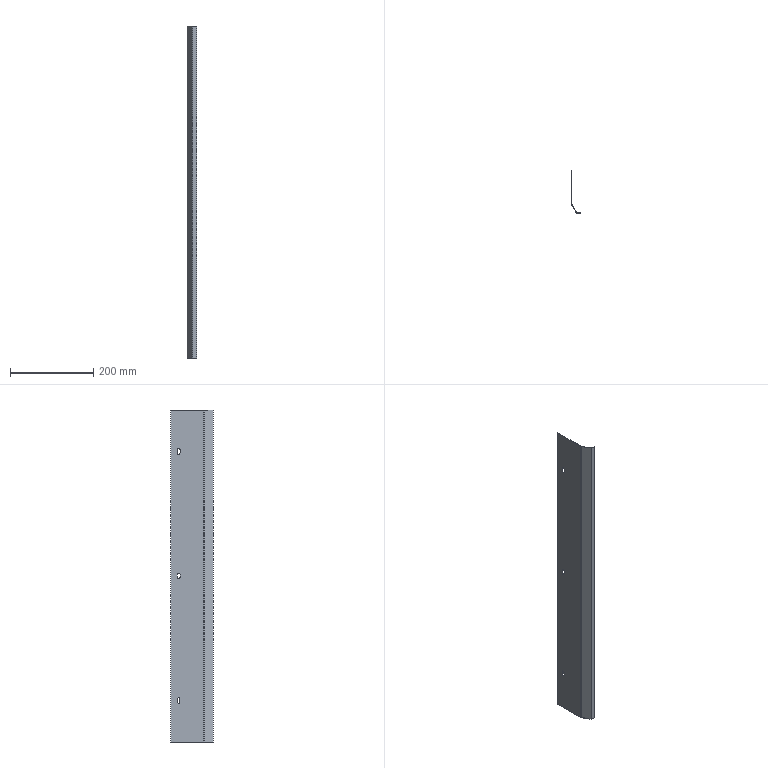Part | SolidWorks | features FlatPattern 1, ICE 1, SMBaseFlange 1, SheetMetal 1 | 1 solid | 37 faces | box 23.5 x 102.651 x 800 mm | volume 92335 mm3 | plane 24 | cylinder 13 | commonest cylinder face diameters 7 x6 6 x3 1 x2 3 x2
STEP:
#1=CARTESIAN_POINT('',(0.,-16.,-296.5));
#2=VERTEX_POINT('',#1);
#3=CARTESIAN_POINT('',(0.,-19.,-293.5));
#4=VERTEX_POINT('',#3);
#5=CARTESIAN_POINT('',(0.,-19.,-296.5));
#6=DIRECTION('',(1.,0.,0.));
#7=DIRECTION('',(0.,1.,0.));
#8=AXIS2_PLACEMENT_3D('',#5,#6,#7);
#9=CIRCLE('',#8,3.);
#10=EDGE_CURVE('',#2,#4,#9,.T.);
#11=ORIENTED_EDGE('',*,*,#10,.T.);
#12=CARTESIAN_POINT('',(-1.,-19.,-293.5));
#13=VERTEX_POINT('',#12);
#14=CARTESIAN_POINT('',(9.,-19.,-293.5));
#15=DIRECTION('',(-1.,0.,0.));
#16=VECTOR('',#15,1000.);
#17=LINE('',#14,#16);
#18=EDGE_CURVE('',#4,#13,#17,.T.);
#19=ORIENTED_EDGE('',*,*,#18,.T.);
#20=CARTESIAN_POINT('',(-1.,-16.,-296.5));
#21=VERTEX_POINT('',#20);
#22=CARTESIAN_POINT('',(-1.,-19.,-296.5));
#23=DIRECTION('',(-1.,0.,0.));
#24=DIRECTION('',(0.,0.,1.));
#25=AXIS2_PLACEMENT_3D('',#22,#23,#24);
#26=CIRCLE('',#25,3.);
#27=EDGE_CURVE('',#13,#21,#26,.T.);
#28=ORIENTED_EDGE('',*,*,#27,.T.);
#29=CARTESIAN_POINT('',(9.,-16.,-296.5));
#30=DIRECTION('',(-1.,0.,0.));
#31=VECTOR('',#30,1000.);
#32=LINE('',#29,#31);
#33=EDGE_CURVE('',#2,#21,#32,.T.);
#34=ORIENTED_EDGE('',*,*,#33,.F.);
#35=EDGE_LOOP('',(#11,#19,#28,#34));
#36=FACE_OUTER_BOUND('',#35,.T.);
#37=CARTESIAN_POINT('',(9.,-19.,-296.5));
#38=DIRECTION('',(-1.,0.,0.));
#39=DIRECTION('',(0.,0.,1.));
#40=AXIS2_PLACEMENT_3D('',#37,#38,#39);
#41=CYLINDRICAL_SURFACE('',#40,3.);
#42=ADVANCED_FACE('',(#36),#41,.F.);
#43=CARTESIAN_POINT('',(0.,-15.5,303.5));
#44=VERTEX_POINT('',#43);
#45=CARTESIAN_POINT('',(0.,-19.,307.));
#46=VERTEX_POINT('',#45);
#47=CARTESIAN_POINT('',(0.,-19.,303.5));
#48=DIRECTION('',(1.,0.,0.));
#49=DIRECTION('',(0.,1.,0.));
#50=AXIS2_PLACEMENT_3D('',#47,#48,#49);
#51=CIRCLE('',#50,3.5);
#52=EDGE_CURVE('',#44,#46,#51,.T.);
#53=ORIENTED_EDGE('',*,*,#52,.T.);
#54=CARTESIAN_POINT('',(-1.,-19.,307.));
#55=VERTEX_POINT('',#54);
#56=CARTESIAN_POINT('',(9.,-19.,307.));
#57=DIRECTION('',(-1.,0.,0.));
#58=VECTOR('',#57,1000.);
#59=LINE('',#56,#58);
#60=EDGE_CURVE('',#46,#55,#59,.T.);
#61=ORIENTED_EDGE('',*,*,#60,.T.);
#62=CARTESIAN_POINT('',(-1.,-15.5,303.5));
#63=VERTEX_POINT('',#62);
#64=CARTESIAN_POINT('',(-1.,-19.,303.5));
#65=DIRECTION('',(-1.,0.,0.));
#66=DIRECTION('',(0.,0.,1.));
#67=AXIS2_PLACEMENT_3D('',#64,#65,#66);
#68=CIRCLE('',#67,3.5);
#69=EDGE_CURVE('',#55,#63,#68,.T.);
#70=ORIENTED_EDGE('',*,*,#69,.T.);
#71=CARTESIAN_POINT('',(9.,-15.5,303.5));
#72=DIRECTION('',(-1.,0.,0.));
#73=VECTOR('',#72,1000.);
#74=LINE('',#71,#73);
#75=EDGE_CURVE('',#44,#63,#74,.T.);
#76=ORIENTED_EDGE('',*,*,#75,.F.);
#77=EDGE_LOOP('',(#53,#61,#70,#76));
#78=FACE_OUTER_BOUND('',#77,.T.);
#79=CARTESIAN_POINT('',(9.,-19.,303.5));
#80=DIRECTION('',(-1.,0.,0.));
#81=DIRECTION('',(0.,0.,1.));
#82=AXIS2_PLACEMENT_3D('',#79,#80,#81);
#83=CYLINDRICAL_SURFACE('',#82,3.5);
#84=ADVANCED_FACE('',(#78),#83,.F.);
#85=CARTESIAN_POINT('',(0.,-15.5,3.5));
#86=VERTEX_POINT('',#85);
#87=CARTESIAN_POINT('',(0.,-19.,7.));
#88=VERTEX_POINT('',#87);
#89=CARTESIAN_POINT('',(0.,-19.,3.5));
#90=DIRECTION('',(1.,0.,0.));
#91=DIRECTION('',(0.,1.,0.));
#92=AXIS2_PLACEMENT_3D('',#89,#90,#91);
#93=CIRCLE('',#92,3.5);
#94=EDGE_CURVE('',#86,#88,#93,.T.);
#95=ORIENTED_EDGE('',*,*,#94,.T.);
#96=CARTESIAN_POINT('',(-1.,-19.,7.));
#97=VERTEX_POINT('',#96);
#98=CARTESIAN_POINT('',(9.,-19.,7.));
#99=DIRECTION('',(-1.,0.,0.));
#100=VECTOR('',#99,1000.);
#101=LINE('',#98,#100);
#102=EDGE_CURVE('',#88,#97,#101,.T.);
#103=ORIENTED_EDGE('',*,*,#102,.T.);
#104=CARTESIAN_POINT('',(-1.,-15.5,3.5));
#105=VERTEX_POINT('',#104);
#106=CARTESIAN_POINT('',(-1.,-19.,3.5));
#107=DIRECTION('',(-1.,0.,0.));
#108=DIRECTION('',(0.,0.,1.));
#109=AXIS2_PLACEMENT_3D('',#106,#107,#108);
#110=CIRCLE('',#109,3.5);
#111=EDGE_CURVE('',#97,#105,#110,.T.);
#112=ORIENTED_EDGE('',*,*,#111,.T.);
#113=CARTESIAN_POINT('',(9.,-15.5,3.5));
#114=DIRECTION('',(-1.,0.,0.));
#115=VECTOR('',#114,1000.);
#116=LINE('',#113,#115);
#117=EDGE_CURVE('',#86,#105,#116,.T.);
#118=ORIENTED_EDGE('',*,*,#117,.F.);
#119=EDGE_LOOP('',(#95,#103,#112,#118));
#120=FACE_OUTER_BOUND('',#119,.T.);
#121=CARTESIAN_POINT('',(9.,-19.,3.5));
#122=DIRECTION('',(-1.,0.,0.));
#123=DIRECTION('',(0.,0.,1.));
#124=AXIS2_PLACEMENT_3D('',#121,#122,#123);
#125=CYLINDRICAL_SURFACE('',#124,3.5);
#126=ADVANCED_FACE('',(#120),#125,.F.);
#127=CARTESIAN_POINT('',(0.06699,-80.116,400.));
#128=VERTEX_POINT('',#127);
#129=CARTESIAN_POINT('',(-0.799,-80.616,400.));
#130=VERTEX_POINT('',#129);
#131=CARTESIAN_POINT('',(0.06699,-80.116,400.));
#132=DIRECTION('',(-0.866,-0.5,0.));
#133=VECTOR('',#132,1000.);
#134=LINE('',#131,#133);
#135=EDGE_CURVE('',#128,#130,#134,.T.);
#136=ORIENTED_EDGE('',*,*,#135,.F.);
#137=CARTESIAN_POINT('',(0.,-79.866,400.));
#138=VERTEX_POINT('',#137);
#139=CARTESIAN_POINT('',(0.5,-79.866,400.));
#140=DIRECTION('',(0.,0.,1.));
#141=DIRECTION('',(-1.,0.,0.));
#142=AXIS2_PLACEMENT_3D('',#139,#140,#141);
#143=CIRCLE('',#142,0.5);
#144=EDGE_CURVE('',#138,#128,#143,.T.);
#145=ORIENTED_EDGE('',*,*,#144,.F.);
#146=CARTESIAN_POINT('',(-1.,-79.866,400.));
#147=VERTEX_POINT('',#146);
#148=CARTESIAN_POINT('',(-1.,-79.866,400.));
#149=DIRECTION('',(1.,0.,0.));
#150=VECTOR('',#149,1000.);
#151=LINE('',#148,#150);
#152=EDGE_CURVE('',#147,#138,#151,.T.);
#153=ORIENTED_EDGE('',*,*,#152,.F.);
#154=CARTESIAN_POINT('',(0.5,-79.866,400.));
#155=DIRECTION('',(0.,0.,1.));
#156=DIRECTION('',(1.,0.,0.));
#157=AXIS2_PLACEMENT_3D('',#154,#155,#156);
#158=CIRCLE('',#157,1.5);
#159=EDGE_CURVE('',#147,#130,#158,.T.);
#160=ORIENTED_EDGE('',*,*,#159,.T.);
#161=EDGE_LOOP('',(#136,#145,#153,#160));
#162=FACE_OUTER_BOUND('',#161,.T.);
#163=CARTESIAN_POINT('',(0.06699,-80.116,400.));
#164=DIRECTION('',(0.,0.,1.));
#165=DIRECTION('',(1.,0.,0.));
#166=AXIS2_PLACEMENT_3D('',#163,#164,#165);
#167=PLANE('',#166);
#168=ADVANCED_FACE('',(#162),#167,.T.);
#169=CARTESIAN_POINT('',(12.356,-101.401,400.));
#170=VERTEX_POINT('',#169);
#171=CARTESIAN_POINT('',(0.,-80.,400.));
#172=DIRECTION('',(0.5,-0.866,0.));
#173=VECTOR('',#172,1000.);
#174=LINE('',#171,#173);
#175=EDGE_CURVE('',#128,#170,#174,.T.);
#176=ORIENTED_EDGE('',*,*,#175,.F.);
#177=ORIENTED_EDGE('',*,*,#135,.T.);
#178=CARTESIAN_POINT('',(11.49,-101.901,400.));
#179=VERTEX_POINT('',#178);
#180=CARTESIAN_POINT('',(-0.866,-80.5,400.));
#181=DIRECTION('',(0.5,-0.866,0.));
#182=VECTOR('',#181,1000.);
#183=LINE('',#180,#182);
#184=EDGE_CURVE('',#130,#179,#183,.T.);
#185=ORIENTED_EDGE('',*,*,#184,.T.);
#186=CARTESIAN_POINT('',(11.49,-101.901,400.));
#187=DIRECTION('',(0.866,0.5,0.));
#188=VECTOR('',#187,1000.);
#189=LINE('',#186,#188);
#190=EDGE_CURVE('',#179,#170,#189,.T.);
#191=ORIENTED_EDGE('',*,*,#190,.T.);
#192=EDGE_LOOP('',(#176,#177,#185,#191));
#193=FACE_OUTER_BOUND('',#192,.T.);
#194=CARTESIAN_POINT('',(-1.,-79.866,400.));
#195=DIRECTION('',(0.,0.,1.));
#196=DIRECTION('',(1.,0.,0.));
#197=AXIS2_PLACEMENT_3D('',#194,#195,#196);
#198=PLANE('',#197);
#199=ADVANCED_FACE('',(#193),#198,.T.);
#200=CARTESIAN_POINT('',(0.,-79.866,-400.));
#201=VERTEX_POINT('',#200);
#202=CARTESIAN_POINT('',(-1.,-79.866,-400.));
#203=VERTEX_POINT('',#202);
#204=CARTESIAN_POINT('',(0.,-79.866,-400.));
#205=DIRECTION('',(-1.,0.,0.));
#206=VECTOR('',#205,1000.);
#207=LINE('',#204,#206);
#208=EDGE_CURVE('',#201,#203,#207,.T.);
#209=ORIENTED_EDGE('',*,*,#208,.F.);
#210=CARTESIAN_POINT('',(0.06699,-80.116,-400.));
#211=VERTEX_POINT('',#210);
#212=CARTESIAN_POINT('',(0.5,-79.866,-400.));
#213=DIRECTION('',(0.,0.,1.));
#214=DIRECTION('',(-1.,0.,0.));
#215=AXIS2_PLACEMENT_3D('',#212,#213,#214);
#216=CIRCLE('',#215,0.5);
#217=EDGE_CURVE('',#201,#211,#216,.T.);
#218=ORIENTED_EDGE('',*,*,#217,.T.);
#219=CARTESIAN_POINT('',(-0.799,-80.616,-400.));
#220=VERTEX_POINT('',#219);
#221=CARTESIAN_POINT('',(-0.799,-80.616,-400.));
#222=DIRECTION('',(0.866,0.5,0.));
#223=VECTOR('',#222,1000.);
#224=LINE('',#221,#223);
#225=EDGE_CURVE('',#220,#211,#224,.T.);
#226=ORIENTED_EDGE('',*,*,#225,.F.);
#227=CARTESIAN_POINT('',(0.5,-79.866,-400.));
#228=DIRECTION('',(0.,0.,1.));
#229=DIRECTION('',(1.,0.,0.));
#230=AXIS2_PLACEMENT_3D('',#227,#228,#229);
#231=CIRCLE('',#230,1.5);
#232=EDGE_CURVE('',#203,#220,#231,.T.);
#233=ORIENTED_EDGE('',*,*,#232,.F.);
#234=EDGE_LOOP('',(#209,#218,#226,#233));
#235=FACE_OUTER_BOUND('',#234,.T.);
#236=CARTESIAN_POINT('',(0.,-79.866,-400.));
#237=DIRECTION('',(0.,0.,-1.));
#238=DIRECTION('',(-1.,0.,0.));
#239=AXIS2_PLACEMENT_3D('',#236,#237,#238);
#240=PLANE('',#239);
#241=ADVANCED_FACE('',(#235),#240,.T.);
#242=CARTESIAN_POINT('',(0.,0.,-400.));
#243=VERTEX_POINT('',#242);
#244=CARTESIAN_POINT('',(0.,0.,-400.));
#245=DIRECTION('',(0.,-1.,0.));
#246=VECTOR('',#245,1000.);
#247=LINE('',#244,#246);
#248=EDGE_CURVE('',#243,#201,#247,.T.);
#249=ORIENTED_EDGE('',*,*,#248,.T.);
#250=ORIENTED_EDGE('',*,*,#208,.T.);
#251=CARTESIAN_POINT('',(-1.,0.,-400.));
#252=VERTEX_POINT('',#251);
#253=CARTESIAN_POINT('',(-1.,0.,-400.));
#254=DIRECTION('',(0.,-1.,0.));
#255=VECTOR('',#254,1000.);
#256=LINE('',#253,#255);
#257=EDGE_CURVE('',#252,#203,#256,.T.);
#258=ORIENTED_EDGE('',*,*,#257,.F.);
#259=CARTESIAN_POINT('',(-1.,0.,-400.));
#260=DIRECTION('',(1.,0.,0.));
#261=VECTOR('',#260,1000.);
#262=LINE('',#259,#261);
#263=EDGE_CURVE('',#252,#243,#262,.T.);
#264=ORIENTED_EDGE('',*,*,#263,.T.);
#265=EDGE_LOOP('',(#249,#250,#258,#264));
#266=FACE_OUTER_BOUND('',#265,.T.);
#267=CARTESIAN_POINT('',(-0.799,-80.616,-400.));
#268=DIRECTION('',(0.,0.,-1.));
#269=DIRECTION('',(-1.,0.,0.));
#270=AXIS2_PLACEMENT_3D('',#267,#268,#269);
#271=PLANE('',#270);
#272=ADVANCED_FACE('',(#266),#271,.T.);
#273=CARTESIAN_POINT('',(12.789,-101.651,400.));
#274=VERTEX_POINT('',#273);
#275=CARTESIAN_POINT('',(12.789,-102.651,400.));
#276=VERTEX_POINT('',#275);
#277=CARTESIAN_POINT('',(12.789,-101.651,400.));
#278=DIRECTION('',(0.,-1.,0.));
#279=VECTOR('',#278,1000.);
#280=LINE('',#277,#279);
#281=EDGE_CURVE('',#274,#276,#280,.T.);
#282=ORIENTED_EDGE('',*,*,#281,.F.);
#283=CARTESIAN_POINT('',(12.789,-101.151,400.));
#284=DIRECTION('',(0.,0.,1.));
#285=DIRECTION('',(-1.,0.,0.));
#286=AXIS2_PLACEMENT_3D('',#283,#284,#285);
#287=CIRCLE('',#286,0.5);
#288=EDGE_CURVE('',#170,#274,#287,.T.);
#289=ORIENTED_EDGE('',*,*,#288,.F.);
#290=ORIENTED_EDGE('',*,*,#190,.F.);
#291=CARTESIAN_POINT('',(12.789,-101.151,400.));
#292=DIRECTION('',(0.,0.,1.));
#293=DIRECTION('',(1.,0.,0.));
#294=AXIS2_PLACEMENT_3D('',#291,#292,#293);
#295=CIRCLE('',#294,1.5);
#296=EDGE_CURVE('',#179,#276,#295,.T.);
#297=ORIENTED_EDGE('',*,*,#296,.T.);
#298=EDGE_LOOP('',(#282,#289,#290,#297));
#299=FACE_OUTER_BOUND('',#298,.T.);
#300=CARTESIAN_POINT('',(12.789,-101.651,400.));
#301=DIRECTION('',(0.,0.,1.));
#302=DIRECTION('',(1.,0.,0.));
#303=AXIS2_PLACEMENT_3D('',#300,#301,#302);
#304=PLANE('',#303);
#305=ADVANCED_FACE('',(#299),#304,.T.);
#306=CARTESIAN_POINT('',(22.5,-101.651,400.));
#307=VERTEX_POINT('',#306);
#308=CARTESIAN_POINT('',(12.5,-101.651,400.));
#309=DIRECTION('',(1.,0.,0.));
#310=VECTOR('',#309,1000.);
#311=LINE('',#308,#310);
#312=EDGE_CURVE('',#274,#307,#311,.T.);
#313=ORIENTED_EDGE('',*,*,#312,.F.);
#314=ORIENTED_EDGE('',*,*,#281,.T.);
#315=CARTESIAN_POINT('',(22.5,-102.651,400.));
#316=VERTEX_POINT('',#315);
#317=CARTESIAN_POINT('',(12.5,-102.651,400.));
#318=DIRECTION('',(1.,0.,0.));
#319=VECTOR('',#318,1000.);
#320=LINE('',#317,#319);
#321=EDGE_CURVE('',#276,#316,#320,.T.);
#322=ORIENTED_EDGE('',*,*,#321,.T.);
#323=CARTESIAN_POINT('',(22.5,-101.651,400.));
#324=DIRECTION('',(0.,-1.,0.));
#325=VECTOR('',#324,1000.);
#326=LINE('',#323,#325);
#327=EDGE_CURVE('',#307,#316,#326,.T.);
#328=ORIENTED_EDGE('',*,*,#327,.F.);
#329=EDGE_LOOP('',(#313,#314,#322,#328));
#330=FACE_OUTER_BOUND('',#329,.T.);
#331=CARTESIAN_POINT('',(11.49,-101.901,400.));
#332=DIRECTION('',(0.,0.,1.));
#333=DIRECTION('',(1.,0.,0.));
#334=AXIS2_PLACEMENT_3D('',#331,#332,#333);
#335=PLANE('',#334);
#336=ADVANCED_FACE('',(#330),#335,.T.);
#337=CARTESIAN_POINT('',(12.356,-101.401,-400.));
#338=VERTEX_POINT('',#337);
#339=CARTESIAN_POINT('',(11.49,-101.901,-400.));
#340=VERTEX_POINT('',#339);
#341=CARTESIAN_POINT('',(12.356,-101.401,-400.));
#342=DIRECTION('',(-0.866,-0.5,0.));
#343=VECTOR('',#342,1000.);
#344=LINE('',#341,#343);
#345=EDGE_CURVE('',#338,#340,#344,.T.);
#346=ORIENTED_EDGE('',*,*,#345,.F.);
#347=CARTESIAN_POINT('',(12.789,-101.651,-400.));
#348=VERTEX_POINT('',#347);
#349=CARTESIAN_POINT('',(12.789,-101.151,-400.));
#350=DIRECTION('',(0.,0.,1.));
#351=DIRECTION('',(-1.,0.,0.));
#352=AXIS2_PLACEMENT_3D('',#349,#350,#351);
#353=CIRCLE('',#352,0.5);
#354=EDGE_CURVE('',#338,#348,#353,.T.);
#355=ORIENTED_EDGE('',*,*,#354,.T.);
#356=CARTESIAN_POINT('',(12.789,-102.651,-400.));
#357=VERTEX_POINT('',#356);
#358=CARTESIAN_POINT('',(12.789,-102.651,-400.));
#359=DIRECTION('',(0.,1.,0.));
#360=VECTOR('',#359,1000.);
#361=LINE('',#358,#360);
#362=EDGE_CURVE('',#357,#348,#361,.T.);
#363=ORIENTED_EDGE('',*,*,#362,.F.);
#364=CARTESIAN_POINT('',(12.789,-101.151,-400.));
#365=DIRECTION('',(0.,0.,1.));
#366=DIRECTION('',(1.,0.,0.));
#367=AXIS2_PLACEMENT_3D('',#364,#365,#366);
#368=CIRCLE('',#367,1.5);
#369=EDGE_CURVE('',#340,#357,#368,.T.);
#370=ORIENTED_EDGE('',*,*,#369,.F.);
#371=EDGE_LOOP('',(#346,#355,#363,#370));
#372=FACE_OUTER_BOUND('',#371,.T.);
#373=CARTESIAN_POINT('',(12.356,-101.401,-400.));
#374=DIRECTION('',(0.,0.,-1.));
#375=DIRECTION('',(-1.,0.,0.));
#376=AXIS2_PLACEMENT_3D('',#373,#374,#375);
#377=PLANE('',#376);
#378=ADVANCED_FACE('',(#372),#377,.T.);
#379=CARTESIAN_POINT('',(0.,-80.,-400.));
#380=DIRECTION('',(0.5,-0.866,0.));
#381=VECTOR('',#380,1000.);
#382=LINE('',#379,#381);
#383=EDGE_CURVE('',#211,#338,#382,.T.);
#384=ORIENTED_EDGE('',*,*,#383,.T.);
#385=ORIENTED_EDGE('',*,*,#345,.T.);
#386=CARTESIAN_POINT('',(-0.866,-80.5,-400.));
#387=DIRECTION('',(0.5,-0.866,0.));
#388=VECTOR('',#387,1000.);
#389=LINE('',#386,#388);
#390=EDGE_CURVE('',#220,#340,#389,.T.);
#391=ORIENTED_EDGE('',*,*,#390,.F.);
#392=ORIENTED_EDGE('',*,*,#225,.T.);
#393=EDGE_LOOP('',(#384,#385,#391,#392));
#394=FACE_OUTER_BOUND('',#393,.T.);
#395=CARTESIAN_POINT('',(12.789,-102.651,-400.));
#396=DIRECTION('',(0.,0.,-1.));
#397=DIRECTION('',(-1.,0.,0.));
#398=AXIS2_PLACEMENT_3D('',#395,#396,#397);
#399=PLANE('',#398);
#400=ADVANCED_FACE('',(#394),#399,.T.);
#401=CARTESIAN_POINT('',(22.5,-102.651,-400.));
#402=VERTEX_POINT('',#401);
#403=CARTESIAN_POINT('',(12.5,-102.651,-400.));
#404=DIRECTION('',(1.,0.,0.));
#405=VECTOR('',#404,1000.);
#406=LINE('',#403,#405);
#407=EDGE_CURVE('',#357,#402,#406,.T.);
#408=ORIENTED_EDGE('',*,*,#407,.T.);
#409=CARTESIAN_POINT('',(22.5,-102.651,400.));
#410=DIRECTION('',(0.,0.,-1.));
#411=VECTOR('',#410,1000.);
#412=LINE('',#409,#411);
#413=EDGE_CURVE('',#316,#402,#412,.T.);
#414=ORIENTED_EDGE('',*,*,#413,.F.);
#415=ORIENTED_EDGE('',*,*,#321,.F.);
#416=CARTESIAN_POINT('',(12.789,-102.651,400.));
#417=DIRECTION('',(0.,0.,-1.));
#418=VECTOR('',#417,1000.);
#419=LINE('',#416,#418);
#420=EDGE_CURVE('',#276,#357,#419,.T.);
#421=ORIENTED_EDGE('',*,*,#420,.T.);
#422=EDGE_LOOP('',(#408,#414,#415,#421));
#423=FACE_OUTER_BOUND('',#422,.T.);
#424=CARTESIAN_POINT('',(12.5,-102.651,400.));
#425=DIRECTION('',(0.,1.,0.));
#426=DIRECTION('',(0.,0.,1.));
#427=AXIS2_PLACEMENT_3D('',#424,#425,#426);
#428=PLANE('',#427);
#429=ADVANCED_FACE('',(#423),#428,.F.);
#430=CARTESIAN_POINT('',(22.5,-101.651,-400.));
#431=VERTEX_POINT('',#430);
#432=CARTESIAN_POINT('',(22.5,-101.651,-400.));
#433=DIRECTION('',(0.,-1.,0.));
#434=VECTOR('',#433,1000.);
#435=LINE('',#432,#434);
#436=EDGE_CURVE('',#431,#402,#435,.T.);
#437=ORIENTED_EDGE('',*,*,#436,.F.);
#438=CARTESIAN_POINT('',(22.5,-101.651,400.));
#439=DIRECTION('',(0.,0.,-1.));
#440=VECTOR('',#439,1000.);
#441=LINE('',#438,#440);
#442=EDGE_CURVE('',#307,#431,#441,.T.);
#443=ORIENTED_EDGE('',*,*,#442,.F.);
#444=ORIENTED_EDGE('',*,*,#327,.T.);
#445=ORIENTED_EDGE('',*,*,#413,.T.);
#446=EDGE_LOOP('',(#437,#443,#444,#445));
#447=FACE_OUTER_BOUND('',#446,.T.);
#448=CARTESIAN_POINT('',(22.5,-101.651,400.));
#449=DIRECTION('',(1.,0.,0.));
#450=DIRECTION('',(0.,0.,-1.));
#451=AXIS2_PLACEMENT_3D('',#448,#449,#450);
#452=PLANE('',#451);
#453=ADVANCED_FACE('',(#447),#452,.T.);
#454=CARTESIAN_POINT('',(12.5,-101.651,-400.));
#455=DIRECTION('',(1.,0.,0.));
#456=VECTOR('',#455,1000.);
#457=LINE('',#454,#456);
#458=EDGE_CURVE('',#348,#431,#457,.T.);
#459=ORIENTED_EDGE('',*,*,#458,.F.);
#460=CARTESIAN_POINT('',(12.789,-101.651,400.));
#461=DIRECTION('',(0.,0.,-1.));
#462=VECTOR('',#461,1000.);
#463=LINE('',#460,#462);
#464=EDGE_CURVE('',#274,#348,#463,.T.);
#465=ORIENTED_EDGE('',*,*,#464,.F.);
#466=ORIENTED_EDGE('',*,*,#312,.T.);
#467=ORIENTED_EDGE('',*,*,#442,.T.);
#468=EDGE_LOOP('',(#459,#465,#466,#467));
#469=FACE_OUTER_BOUND('',#468,.T.);
#470=CARTESIAN_POINT('',(12.5,-101.651,400.));
#471=DIRECTION('',(0.,1.,0.));
#472=DIRECTION('',(0.,0.,1.));
#473=AXIS2_PLACEMENT_3D('',#470,#471,#472);
#474=PLANE('',#473);
#475=ADVANCED_FACE('',(#469),#474,.T.);
#476=ORIENTED_EDGE('',*,*,#354,.F.);
#477=CARTESIAN_POINT('',(12.356,-101.401,400.));
#478=DIRECTION('',(0.,0.,-1.));
#479=VECTOR('',#478,1000.);
#480=LINE('',#477,#479);
#481=EDGE_CURVE('',#170,#338,#480,.T.);
#482=ORIENTED_EDGE('',*,*,#481,.F.);
#483=ORIENTED_EDGE('',*,*,#288,.T.);
#484=ORIENTED_EDGE('',*,*,#464,.T.);
#485=EDGE_LOOP('',(#476,#482,#483,#484));
#486=FACE_OUTER_BOUND('',#485,.T.);
#487=CARTESIAN_POINT('',(12.789,-101.151,400.));
#488=DIRECTION('',(0.,0.,-1.));
#489=DIRECTION('',(-1.,0.,0.));
#490=AXIS2_PLACEMENT_3D('',#487,#488,#489);
#491=CYLINDRICAL_SURFACE('',#490,0.5);
#492=ADVANCED_FACE('',(#486),#491,.F.);
#493=ORIENTED_EDGE('',*,*,#383,.F.);
#494=CARTESIAN_POINT('',(0.06699,-80.116,400.));
#495=DIRECTION('',(0.,0.,-1.));
#496=VECTOR('',#495,1000.);
#497=LINE('',#494,#496);
#498=EDGE_CURVE('',#128,#211,#497,.T.);
#499=ORIENTED_EDGE('',*,*,#498,.F.);
#500=ORIENTED_EDGE('',*,*,#175,.T.);
#501=ORIENTED_EDGE('',*,*,#481,.T.);
#502=EDGE_LOOP('',(#493,#499,#500,#501));
#503=FACE_OUTER_BOUND('',#502,.T.);
#504=CARTESIAN_POINT('',(0.,-80.,400.));
#505=DIRECTION('',(0.866,0.5,0.));
#506=DIRECTION('',(-0.5,0.866,0.));
#507=AXIS2_PLACEMENT_3D('',#504,#505,#506);
#508=PLANE('',#507);
#509=ADVANCED_FACE('',(#503),#508,.T.);
#510=ORIENTED_EDGE('',*,*,#217,.F.);
#511=CARTESIAN_POINT('',(0.,-79.866,400.));
#512=DIRECTION('',(0.,0.,-1.));
#513=VECTOR('',#512,1000.);
#514=LINE('',#511,#513);
#515=EDGE_CURVE('',#138,#201,#514,.T.);
#516=ORIENTED_EDGE('',*,*,#515,.F.);
#517=ORIENTED_EDGE('',*,*,#144,.T.);
#518=ORIENTED_EDGE('',*,*,#498,.T.);
#519=EDGE_LOOP('',(#510,#516,#517,#518));
#520=FACE_OUTER_BOUND('',#519,.T.);
#521=CARTESIAN_POINT('',(0.5,-79.866,400.));
#522=DIRECTION('',(0.,0.,-1.));
#523=DIRECTION('',(-1.,0.,0.));
#524=AXIS2_PLACEMENT_3D('',#521,#522,#523);
#525=CYLINDRICAL_SURFACE('',#524,0.5);
#526=ADVANCED_FACE('',(#520),#525,.F.);
#527=CARTESIAN_POINT('',(0.,-22.,-303.5));
#528=VERTEX_POINT('',#527);
#529=CARTESIAN_POINT('',(0.,-16.,-303.5));
#530=VERTEX_POINT('',#529);
#531=CARTESIAN_POINT('',(0.,-19.,-303.5));
#532=DIRECTION('',(1.,0.,0.));
#533=DIRECTION('',(0.,1.,0.));
#534=AXIS2_PLACEMENT_3D('',#531,#532,#533);
#535=CIRCLE('',#534,3.);
#536=EDGE_CURVE('',#528,#530,#535,.T.);
#537=ORIENTED_EDGE('',*,*,#536,.F.);
#538=CARTESIAN_POINT('',(0.,-22.,-296.5));
#539=VERTEX_POINT('',#538);
#540=CARTESIAN_POINT('',(0.,-22.,400.));
#541=DIRECTION('',(0.,0.,-1.));
#542=VECTOR('',#541,1000.);
#543=LINE('',#540,#542);
#544=EDGE_CURVE('',#539,#528,#543,.T.);
#545=ORIENTED_EDGE('',*,*,#544,.F.);
#546=CARTESIAN_POINT('',(0.,-19.,-296.5));
#547=DIRECTION('',(1.,0.,0.));
#548=DIRECTION('',(0.,1.,0.));
#549=AXIS2_PLACEMENT_3D('',#546,#547,#548);
#550=CIRCLE('',#549,3.);
#551=EDGE_CURVE('',#4,#539,#550,.T.);
#552=ORIENTED_EDGE('',*,*,#551,.F.);
#553=ORIENTED_EDGE('',*,*,#10,.F.);
#554=CARTESIAN_POINT('',(0.,-16.,400.));
#555=DIRECTION('',(0.,0.,1.));
#556=VECTOR('',#555,1000.);
#557=LINE('',#554,#556);
#558=EDGE_CURVE('',#530,#2,#557,.T.);
#559=ORIENTED_EDGE('',*,*,#558,.F.);
#560=EDGE_LOOP('',(#537,#545,#552,#553,#559));
#561=FACE_BOUND('',#560,.T.);
#562=CARTESIAN_POINT('',(0.,-22.5,296.5));
#563=VERTEX_POINT('',#562);
#564=CARTESIAN_POINT('',(0.,-15.5,296.5));
#565=VERTEX_POINT('',#564);
#566=CARTESIAN_POINT('',(0.,-19.,296.5));
#567=DIRECTION('',(1.,0.,0.));
#568=DIRECTION('',(0.,1.,0.));
#569=AXIS2_PLACEMENT_3D('',#566,#567,#568);
#570=CIRCLE('',#569,3.5);
#571=EDGE_CURVE('',#563,#565,#570,.T.);
#572=ORIENTED_EDGE('',*,*,#571,.F.);
#573=CARTESIAN_POINT('',(0.,-22.5,303.5));
#574=VERTEX_POINT('',#573);
#575=CARTESIAN_POINT('',(0.,-22.5,400.));
#576=DIRECTION('',(0.,0.,-1.));
#577=VECTOR('',#576,1000.);
#578=LINE('',#575,#577);
#579=EDGE_CURVE('',#574,#563,#578,.T.);
#580=ORIENTED_EDGE('',*,*,#579,.F.);
#581=CARTESIAN_POINT('',(0.,-19.,303.5));
#582=DIRECTION('',(1.,0.,0.));
#583=DIRECTION('',(0.,1.,0.));
#584=AXIS2_PLACEMENT_3D('',#581,#582,#583);
#585=CIRCLE('',#584,3.5);
#586=EDGE_CURVE('',#46,#574,#585,.T.);
#587=ORIENTED_EDGE('',*,*,#586,.F.);
#588=ORIENTED_EDGE('',*,*,#52,.F.);
#589=CARTESIAN_POINT('',(0.,-15.5,400.));
#590=DIRECTION('',(0.,0.,1.));
#591=VECTOR('',#590,1000.);
#592=LINE('',#589,#591);
#593=EDGE_CURVE('',#565,#44,#592,.T.);
#594=ORIENTED_EDGE('',*,*,#593,.F.);
#595=EDGE_LOOP('',(#572,#580,#587,#588,#594));
#596=FACE_BOUND('',#595,.T.);
#597=CARTESIAN_POINT('',(0.,-22.5,-3.5));
#598=VERTEX_POINT('',#597);
#599=CARTESIAN_POINT('',(0.,-15.5,-3.5));
#600=VERTEX_POINT('',#599);
#601=CARTESIAN_POINT('',(0.,-19.,-3.5));
#602=DIRECTION('',(1.,0.,0.));
#603=DIRECTION('',(0.,1.,0.));
#604=AXIS2_PLACEMENT_3D('',#601,#602,#603);
#605=CIRCLE('',#604,3.5);
#606=EDGE_CURVE('',#598,#600,#605,.T.);
#607=ORIENTED_EDGE('',*,*,#606,.F.);
#608=CARTESIAN_POINT('',(0.,-22.5,3.5));
#609=VERTEX_POINT('',#608);
#610=CARTESIAN_POINT('',(0.,-22.5,400.));
#611=DIRECTION('',(0.,0.,-1.));
#612=VECTOR('',#611,1000.);
#613=LINE('',#610,#612);
#614=EDGE_CURVE('',#609,#598,#613,.T.);
#615=ORIENTED_EDGE('',*,*,#614,.F.);
#616=CARTESIAN_POINT('',(0.,-19.,3.5));
#617=DIRECTION('',(1.,0.,0.));
#618=DIRECTION('',(0.,1.,0.));
#619=AXIS2_PLACEMENT_3D('',#616,#617,#618);
#620=CIRCLE('',#619,3.5);
#621=EDGE_CURVE('',#88,#609,#620,.T.);
#622=ORIENTED_EDGE('',*,*,#621,.F.);
#623=ORIENTED_EDGE('',*,*,#94,.F.);
#624=CARTESIAN_POINT('',(0.,-15.5,400.));
#625=DIRECTION('',(0.,0.,1.));
#626=VECTOR('',#625,1000.);
#627=LINE('',#624,#626);
#628=EDGE_CURVE('',#600,#86,#627,.T.);
#629=ORIENTED_EDGE('',*,*,#628,.F.);
#630=EDGE_LOOP('',(#607,#615,#622,#623,#629));
#631=FACE_BOUND('',#630,.T.);
#632=ORIENTED_EDGE('',*,*,#248,.F.);
#633=CARTESIAN_POINT('',(0.,0.,400.));
#634=VERTEX_POINT('',#633);
#635=CARTESIAN_POINT('',(0.,0.,400.));
#636=DIRECTION('',(0.,0.,-1.));
#637=VECTOR('',#636,1000.);
#638=LINE('',#635,#637);
#639=EDGE_CURVE('',#634,#243,#638,.T.);
#640=ORIENTED_EDGE('',*,*,#639,.F.);
#641=CARTESIAN_POINT('',(0.,0.,400.));
#642=DIRECTION('',(0.,-1.,0.));
#643=VECTOR('',#642,1000.);
#644=LINE('',#641,#643);
#645=EDGE_CURVE('',#634,#138,#644,.T.);
#646=ORIENTED_EDGE('',*,*,#645,.T.);
#647=ORIENTED_EDGE('',*,*,#515,.T.);
#648=EDGE_LOOP('',(#632,#640,#646,#647));
#649=FACE_OUTER_BOUND('',#648,.T.);
#650=CARTESIAN_POINT('',(0.,0.,400.));
#651=DIRECTION('',(1.,0.,0.));
#652=DIRECTION('',(0.,1.,0.));
#653=AXIS2_PLACEMENT_3D('',#650,#651,#652);
#654=PLANE('',#653);
#655=ADVANCED_FACE('',(#561,#596,#631,#649),#654,.T.);
#656=ORIENTED_EDGE('',*,*,#263,.F.);
#657=CARTESIAN_POINT('',(-1.,0.,400.));
#658=VERTEX_POINT('',#657);
#659=CARTESIAN_POINT('',(-1.,0.,400.));
#660=DIRECTION('',(0.,0.,-1.));
#661=VECTOR('',#660,1000.);
#662=LINE('',#659,#661);
#663=EDGE_CURVE('',#658,#252,#662,.T.);
#664=ORIENTED_EDGE('',*,*,#663,.F.);
#665=CARTESIAN_POINT('',(-1.,0.,400.));
#666=DIRECTION('',(1.,0.,0.));
#667=VECTOR('',#666,1000.);
#668=LINE('',#665,#667);
#669=EDGE_CURVE('',#658,#634,#668,.T.);
#670=ORIENTED_EDGE('',*,*,#669,.T.);
#671=ORIENTED_EDGE('',*,*,#639,.T.);
#672=EDGE_LOOP('',(#656,#664,#670,#671));
#673=FACE_OUTER_BOUND('',#672,.T.);
#674=CARTESIAN_POINT('',(-1.,0.,400.));
#675=DIRECTION('',(0.,1.,0.));
#676=DIRECTION('',(-1.,0.,0.));
#677=AXIS2_PLACEMENT_3D('',#674,#675,#676);
#678=PLANE('',#677);
#679=ADVANCED_FACE('',(#673),#678,.T.);
#680=CARTESIAN_POINT('',(-1.,-22.,-303.5));
#681=VERTEX_POINT('',#680);
#682=CARTESIAN_POINT('',(-1.,-22.,-296.5));
#683=VERTEX_POINT('',#682);
#684=CARTESIAN_POINT('',(-1.,-22.,-303.5));
#685=DIRECTION('',(0.,0.,1.));
#686=VECTOR('',#685,1000.);
#687=LINE('',#684,#686);
#688=EDGE_CURVE('',#681,#683,#687,.T.);
#689=ORIENTED_EDGE('',*,*,#688,.F.);
#690=CARTESIAN_POINT('',(-1.,-16.,-303.5));
#691=VERTEX_POINT('',#690);
#692=CARTESIAN_POINT('',(-1.,-19.,-303.5));
#693=DIRECTION('',(-1.,0.,0.));
#694=DIRECTION('',(0.,0.,1.));
#695=AXIS2_PLACEMENT_3D('',#692,#693,#694);
#696=CIRCLE('',#695,3.);
#697=EDGE_CURVE('',#691,#681,#696,.T.);
#698=ORIENTED_EDGE('',*,*,#697,.F.);
#699=CARTESIAN_POINT('',(-1.,-16.,-303.5));
#700=DIRECTION('',(0.,0.,-1.));
#701=VECTOR('',#700,1000.);
#702=LINE('',#699,#701);
#703=EDGE_CURVE('',#21,#691,#702,.T.);
#704=ORIENTED_EDGE('',*,*,#703,.F.);
#705=ORIENTED_EDGE('',*,*,#27,.F.);
#706=CARTESIAN_POINT('',(-1.,-19.,-296.5));
#707=DIRECTION('',(-1.,0.,0.));
#708=DIRECTION('',(0.,0.,1.));
#709=AXIS2_PLACEMENT_3D('',#706,#707,#708);
#710=CIRCLE('',#709,3.);
#711=EDGE_CURVE('',#683,#13,#710,.T.);
#712=ORIENTED_EDGE('',*,*,#711,.F.);
#713=EDGE_LOOP('',(#689,#698,#704,#705,#712));
#714=FACE_BOUND('',#713,.T.);
#715=CARTESIAN_POINT('',(-1.,-22.5,296.5));
#716=VERTEX_POINT('',#715);
#717=CARTESIAN_POINT('',(-1.,-22.5,303.5));
#718=VERTEX_POINT('',#717);
#719=CARTESIAN_POINT('',(-1.,-22.5,296.5));
#720=DIRECTION('',(0.,0.,1.));
#721=VECTOR('',#720,1000.);
#722=LINE('',#719,#721);
#723=EDGE_CURVE('',#716,#718,#722,.T.);
#724=ORIENTED_EDGE('',*,*,#723,.F.);
#725=CARTESIAN_POINT('',(-1.,-15.5,296.5));
#726=VERTEX_POINT('',#725);
#727=CARTESIAN_POINT('',(-1.,-19.,296.5));
#728=DIRECTION('',(-1.,0.,0.));
#729=DIRECTION('',(0.,0.,1.));
#730=AXIS2_PLACEMENT_3D('',#727,#728,#729);
#731=CIRCLE('',#730,3.5);
#732=EDGE_CURVE('',#726,#716,#731,.T.);
#733=ORIENTED_EDGE('',*,*,#732,.F.);
#734=CARTESIAN_POINT('',(-1.,-15.5,296.5));
#735=DIRECTION('',(0.,0.,-1.));
#736=VECTOR('',#735,1000.);
#737=LINE('',#734,#736);
#738=EDGE_CURVE('',#63,#726,#737,.T.);
#739=ORIENTED_EDGE('',*,*,#738,.F.);
#740=ORIENTED_EDGE('',*,*,#69,.F.);
#741=CARTESIAN_POINT('',(-1.,-19.,303.5));
#742=DIRECTION('',(-1.,0.,0.));
#743=DIRECTION('',(0.,0.,1.));
#744=AXIS2_PLACEMENT_3D('',#741,#742,#743);
#745=CIRCLE('',#744,3.5);
#746=EDGE_CURVE('',#718,#55,#745,.T.);
#747=ORIENTED_EDGE('',*,*,#746,.F.);
#748=EDGE_LOOP('',(#724,#733,#739,#740,#747));
#749=FACE_BOUND('',#748,.T.);
#750=CARTESIAN_POINT('',(-1.,-22.5,-3.5));
#751=VERTEX_POINT('',#750);
#752=CARTESIAN_POINT('',(-1.,-22.5,3.5));
#753=VERTEX_POINT('',#752);
#754=CARTESIAN_POINT('',(-1.,-22.5,-3.5));
#755=DIRECTION('',(0.,0.,1.));
#756=VECTOR('',#755,1000.);
#757=LINE('',#754,#756);
#758=EDGE_CURVE('',#751,#753,#757,.T.);
#759=ORIENTED_EDGE('',*,*,#758,.F.);
#760=CARTESIAN_POINT('',(-1.,-15.5,-3.5));
#761=VERTEX_POINT('',#760);
#762=CARTESIAN_POINT('',(-1.,-19.,-3.5));
#763=DIRECTION('',(-1.,0.,0.));
#764=DIRECTION('',(0.,0.,1.));
#765=AXIS2_PLACEMENT_3D('',#762,#763,#764);
#766=CIRCLE('',#765,3.5);
#767=EDGE_CURVE('',#761,#751,#766,.T.);
#768=ORIENTED_EDGE('',*,*,#767,.F.);
#769=CARTESIAN_POINT('',(-1.,-15.5,-3.5));
#770=DIRECTION('',(0.,0.,-1.));
#771=VECTOR('',#770,1000.);
#772=LINE('',#769,#771);
#773=EDGE_CURVE('',#105,#761,#772,.T.);
#774=ORIENTED_EDGE('',*,*,#773,.F.);
#775=ORIENTED_EDGE('',*,*,#111,.F.);
#776=CARTESIAN_POINT('',(-1.,-19.,3.5));
#777=DIRECTION('',(-1.,0.,0.));
#778=DIRECTION('',(0.,0.,1.));
#779=AXIS2_PLACEMENT_3D('',#776,#777,#778);
#780=CIRCLE('',#779,3.5);
#781=EDGE_CURVE('',#753,#97,#780,.T.);
#782=ORIENTED_EDGE('',*,*,#781,.F.);
#783=EDGE_LOOP('',(#759,#768,#774,#775,#782));
#784=FACE_BOUND('',#783,.T.);
#785=ORIENTED_EDGE('',*,*,#257,.T.);
#786=CARTESIAN_POINT('',(-1.,-79.866,400.));
#787=DIRECTION('',(0.,0.,-1.));
#788=VECTOR('',#787,1000.);
#789=LINE('',#786,#788);
#790=EDGE_CURVE('',#147,#203,#789,.T.);
#791=ORIENTED_EDGE('',*,*,#790,.F.);
#792=CARTESIAN_POINT('',(-1.,0.,400.));
#793=DIRECTION('',(0.,-1.,0.));
#794=VECTOR('',#793,1000.);
#795=LINE('',#792,#794);
#796=EDGE_CURVE('',#658,#147,#795,.T.);
#797=ORIENTED_EDGE('',*,*,#796,.F.);
#798=ORIENTED_EDGE('',*,*,#663,.T.);
#799=EDGE_LOOP('',(#785,#791,#797,#798));
#800=FACE_OUTER_BOUND('',#799,.T.);
#801=CARTESIAN_POINT('',(-1.,0.,400.));
#802=DIRECTION('',(1.,0.,0.));
#803=DIRECTION('',(0.,1.,0.));
#804=AXIS2_PLACEMENT_3D('',#801,#802,#803);
#805=PLANE('',#804);
#806=ADVANCED_FACE('',(#714,#749,#784,#800),#805,.F.);
#807=ORIENTED_EDGE('',*,*,#232,.T.);
#808=CARTESIAN_POINT('',(-0.799,-80.616,400.));
#809=DIRECTION('',(0.,0.,-1.));
#810=VECTOR('',#809,1000.);
#811=LINE('',#808,#810);
#812=EDGE_CURVE('',#130,#220,#811,.T.);
#813=ORIENTED_EDGE('',*,*,#812,.F.);
#814=ORIENTED_EDGE('',*,*,#159,.F.);
#815=ORIENTED_EDGE('',*,*,#790,.T.);
#816=EDGE_LOOP('',(#807,#813,#814,#815));
#817=FACE_OUTER_BOUND('',#816,.T.);
#818=CARTESIAN_POINT('',(0.5,-79.866,400.));
#819=DIRECTION('',(0.,0.,-1.));
#820=DIRECTION('',(-1.,0.,0.));
#821=AXIS2_PLACEMENT_3D('',#818,#819,#820);
#822=CYLINDRICAL_SURFACE('',#821,1.5);
#823=ADVANCED_FACE('',(#817),#822,.T.);
#824=ORIENTED_EDGE('',*,*,#390,.T.);
#825=CARTESIAN_POINT('',(11.49,-101.901,400.));
#826=DIRECTION('',(0.,0.,-1.));
#827=VECTOR('',#826,1000.);
#828=LINE('',#825,#827);
#829=EDGE_CURVE('',#179,#340,#828,.T.);
#830=ORIENTED_EDGE('',*,*,#829,.F.);
#831=ORIENTED_EDGE('',*,*,#184,.F.);
#832=ORIENTED_EDGE('',*,*,#812,.T.);
#833=EDGE_LOOP('',(#824,#830,#831,#832));
#834=FACE_OUTER_BOUND('',#833,.T.);
#835=CARTESIAN_POINT('',(-0.866,-80.5,400.));
#836=DIRECTION('',(0.866,0.5,0.));
#837=DIRECTION('',(-0.5,0.866,0.));
#838=AXIS2_PLACEMENT_3D('',#835,#836,#837);
#839=PLANE('',#838);
#840=ADVANCED_FACE('',(#834),#839,.F.);
#841=ORIENTED_EDGE('',*,*,#369,.T.);
#842=ORIENTED_EDGE('',*,*,#420,.F.);
#843=ORIENTED_EDGE('',*,*,#296,.F.);
#844=ORIENTED_EDGE('',*,*,#829,.T.);
#845=EDGE_LOOP('',(#841,#842,#843,#844));
#846=FACE_OUTER_BOUND('',#845,.T.);
#847=CARTESIAN_POINT('',(12.789,-101.151,400.));
#848=DIRECTION('',(0.,0.,-1.));
#849=DIRECTION('',(-1.,0.,0.));
#850=AXIS2_PLACEMENT_3D('',#847,#848,#849);
#851=CYLINDRICAL_SURFACE('',#850,1.5);
#852=ADVANCED_FACE('',(#846),#851,.T.);
#853=ORIENTED_EDGE('',*,*,#796,.T.);
#854=ORIENTED_EDGE('',*,*,#152,.T.);
#855=ORIENTED_EDGE('',*,*,#645,.F.);
#856=ORIENTED_EDGE('',*,*,#669,.F.);
#857=EDGE_LOOP('',(#853,#854,#855,#856));
#858=FACE_OUTER_BOUND('',#857,.T.);
#859=CARTESIAN_POINT('',(12.789,-101.151,400.));
#860=DIRECTION('',(0.,0.,-1.));
#861=DIRECTION('',(-1.,0.,0.));
#862=AXIS2_PLACEMENT_3D('',#859,#860,#861);
#863=PLANE('',#862);
#864=ADVANCED_FACE('',(#858),#863,.F.);
#865=ORIENTED_EDGE('',*,*,#407,.F.);
#866=ORIENTED_EDGE('',*,*,#362,.T.);
#867=ORIENTED_EDGE('',*,*,#458,.T.);
#868=ORIENTED_EDGE('',*,*,#436,.T.);
#869=EDGE_LOOP('',(#865,#866,#867,#868));
#870=FACE_OUTER_BOUND('',#869,.T.);
#871=CARTESIAN_POINT('',(12.789,-101.151,-400.));
#872=DIRECTION('',(0.,0.,-1.));
#873=DIRECTION('',(-1.,0.,0.));
#874=AXIS2_PLACEMENT_3D('',#871,#872,#873);
#875=PLANE('',#874);
#876=ADVANCED_FACE('',(#870),#875,.T.);
#877=ORIENTED_EDGE('',*,*,#606,.T.);
#878=CARTESIAN_POINT('',(9.,-15.5,-3.5));
#879=DIRECTION('',(-1.,0.,0.));
#880=VECTOR('',#879,1000.);
#881=LINE('',#878,#880);
#882=EDGE_CURVE('',#600,#761,#881,.T.);
#883=ORIENTED_EDGE('',*,*,#882,.T.);
#884=ORIENTED_EDGE('',*,*,#767,.T.);
#885=CARTESIAN_POINT('',(9.,-22.5,-3.5));
#886=DIRECTION('',(-1.,0.,0.));
#887=VECTOR('',#886,1000.);
#888=LINE('',#885,#887);
#889=EDGE_CURVE('',#598,#751,#888,.T.);
#890=ORIENTED_EDGE('',*,*,#889,.F.);
#891=EDGE_LOOP('',(#877,#883,#884,#890));
#892=FACE_OUTER_BOUND('',#891,.T.);
#893=CARTESIAN_POINT('',(9.,-19.,-3.5));
#894=DIRECTION('',(-1.,0.,0.));
#895=DIRECTION('',(0.,0.,1.));
#896=AXIS2_PLACEMENT_3D('',#893,#894,#895);
#897=CYLINDRICAL_SURFACE('',#896,3.5);
#898=ADVANCED_FACE('',(#892),#897,.F.);
#899=ORIENTED_EDGE('',*,*,#628,.T.);
#900=ORIENTED_EDGE('',*,*,#117,.T.);
#901=ORIENTED_EDGE('',*,*,#773,.T.);
#902=ORIENTED_EDGE('',*,*,#882,.F.);
#903=EDGE_LOOP('',(#899,#900,#901,#902));
#904=FACE_OUTER_BOUND('',#903,.T.);
#905=CARTESIAN_POINT('',(9.,-15.5,-3.5));
#906=DIRECTION('',(0.,1.,0.));
#907=DIRECTION('',(0.,0.,1.));
#908=AXIS2_PLACEMENT_3D('',#905,#906,#907);
#909=PLANE('',#908);
#910=ADVANCED_FACE('',(#904),#909,.F.);
#911=ORIENTED_EDGE('',*,*,#102,.F.);
#912=ORIENTED_EDGE('',*,*,#621,.T.);
#913=CARTESIAN_POINT('',(9.,-22.5,3.5));
#914=DIRECTION('',(-1.,0.,0.));
#915=VECTOR('',#914,1000.);
#916=LINE('',#913,#915);
#917=EDGE_CURVE('',#609,#753,#916,.T.);
#918=ORIENTED_EDGE('',*,*,#917,.T.);
#919=ORIENTED_EDGE('',*,*,#781,.T.);
#920=EDGE_LOOP('',(#911,#912,#918,#919));
#921=FACE_OUTER_BOUND('',#920,.T.);
#922=CARTESIAN_POINT('',(9.,-19.,3.5));
#923=DIRECTION('',(-1.,0.,0.));
#924=DIRECTION('',(0.,0.,1.));
#925=AXIS2_PLACEMENT_3D('',#922,#923,#924);
#926=CYLINDRICAL_SURFACE('',#925,3.5);
#927=ADVANCED_FACE('',(#921),#926,.F.);
#928=ORIENTED_EDGE('',*,*,#614,.T.);
#929=ORIENTED_EDGE('',*,*,#889,.T.);
#930=ORIENTED_EDGE('',*,*,#758,.T.);
#931=ORIENTED_EDGE('',*,*,#917,.F.);
#932=EDGE_LOOP('',(#928,#929,#930,#931));
#933=FACE_OUTER_BOUND('',#932,.T.);
#934=CARTESIAN_POINT('',(9.,-22.5,-3.5));
#935=DIRECTION('',(0.,-1.,0.));
#936=DIRECTION('',(0.,0.,-1.));
#937=AXIS2_PLACEMENT_3D('',#934,#935,#936);
#938=PLANE('',#937);
#939=ADVANCED_FACE('',(#933),#938,.F.);
#940=ORIENTED_EDGE('',*,*,#571,.T.);
#941=CARTESIAN_POINT('',(9.,-15.5,296.5));
#942=DIRECTION('',(-1.,0.,0.));
#943=VECTOR('',#942,1000.);
#944=LINE('',#941,#943);
#945=EDGE_CURVE('',#565,#726,#944,.T.);
#946=ORIENTED_EDGE('',*,*,#945,.T.);
#947=ORIENTED_EDGE('',*,*,#732,.T.);
#948=CARTESIAN_POINT('',(9.,-22.5,296.5));
#949=DIRECTION('',(-1.,0.,0.));
#950=VECTOR('',#949,1000.);
#951=LINE('',#948,#950);
#952=EDGE_CURVE('',#563,#716,#951,.T.);
#953=ORIENTED_EDGE('',*,*,#952,.F.);
#954=EDGE_LOOP('',(#940,#946,#947,#953));
#955=FACE_OUTER_BOUND('',#954,.T.);
#956=CARTESIAN_POINT('',(9.,-19.,296.5));
#957=DIRECTION('',(-1.,0.,0.));
#958=DIRECTION('',(0.,0.,1.));
#959=AXIS2_PLACEMENT_3D('',#956,#957,#958);
#960=CYLINDRICAL_SURFACE('',#959,3.5);
#961=ADVANCED_FACE('',(#955),#960,.F.);
#962=ORIENTED_EDGE('',*,*,#593,.T.);
#963=ORIENTED_EDGE('',*,*,#75,.T.);
#964=ORIENTED_EDGE('',*,*,#738,.T.);
#965=ORIENTED_EDGE('',*,*,#945,.F.);
#966=EDGE_LOOP('',(#962,#963,#964,#965));
#967=FACE_OUTER_BOUND('',#966,.T.);
#968=CARTESIAN_POINT('',(9.,-15.5,296.5));
#969=DIRECTION('',(0.,1.,0.));
#970=DIRECTION('',(0.,0.,1.));
#971=AXIS2_PLACEMENT_3D('',#968,#969,#970);
#972=PLANE('',#971);
#973=ADVANCED_FACE('',(#967),#972,.F.);
#974=ORIENTED_EDGE('',*,*,#60,.F.);
#975=ORIENTED_EDGE('',*,*,#586,.T.);
#976=CARTESIAN_POINT('',(9.,-22.5,303.5));
#977=DIRECTION('',(-1.,0.,0.));
#978=VECTOR('',#977,1000.);
#979=LINE('',#976,#978);
#980=EDGE_CURVE('',#574,#718,#979,.T.);
#981=ORIENTED_EDGE('',*,*,#980,.T.);
#982=ORIENTED_EDGE('',*,*,#746,.T.);
#983=EDGE_LOOP('',(#974,#975,#981,#982));
#984=FACE_OUTER_BOUND('',#983,.T.);
#985=CARTESIAN_POINT('',(9.,-19.,303.5));
#986=DIRECTION('',(-1.,0.,0.));
#987=DIRECTION('',(0.,0.,1.));
#988=AXIS2_PLACEMENT_3D('',#985,#986,#987);
#989=CYLINDRICAL_SURFACE('',#988,3.5);
#990=ADVANCED_FACE('',(#984),#989,.F.);
#991=ORIENTED_EDGE('',*,*,#579,.T.);
#992=ORIENTED_EDGE('',*,*,#952,.T.);
#993=ORIENTED_EDGE('',*,*,#723,.T.);
#994=ORIENTED_EDGE('',*,*,#980,.F.);
#995=EDGE_LOOP('',(#991,#992,#993,#994));
#996=FACE_OUTER_BOUND('',#995,.T.);
#997=CARTESIAN_POINT('',(9.,-22.5,296.5));
#998=DIRECTION('',(0.,-1.,0.));
#999=DIRECTION('',(0.,0.,-1.));
#1000=AXIS2_PLACEMENT_3D('',#997,#998,#999);
#1001=PLANE('',#1000);
#1002=ADVANCED_FACE('',(#996),#1001,.F.);
#1003=ORIENTED_EDGE('',*,*,#536,.T.);
#1004=CARTESIAN_POINT('',(9.,-16.,-303.5));
#1005=DIRECTION('',(-1.,0.,0.));
#1006=VECTOR('',#1005,1000.);
#1007=LINE('',#1004,#1006);
#1008=EDGE_CURVE('',#530,#691,#1007,.T.);
#1009=ORIENTED_EDGE('',*,*,#1008,.T.);
#1010=ORIENTED_EDGE('',*,*,#697,.T.);
#1011=CARTESIAN_POINT('',(9.,-22.,-303.5));
#1012=DIRECTION('',(-1.,0.,0.));
#1013=VECTOR('',#1012,1000.);
#1014=LINE('',#1011,#1013);
#1015=EDGE_CURVE('',#528,#681,#1014,.T.);
#1016=ORIENTED_EDGE('',*,*,#1015,.F.);
#1017=EDGE_LOOP('',(#1003,#1009,#1010,#1016));
#1018=FACE_OUTER_BOUND('',#1017,.T.);
#1019=CARTESIAN_POINT('',(9.,-19.,-303.5));
#1020=DIRECTION('',(-1.,0.,0.));
#1021=DIRECTION('',(0.,0.,1.));
#1022=AXIS2_PLACEMENT_3D('',#1019,#1020,#1021);
#1023=CYLINDRICAL_SURFACE('',#1022,3.);
#1024=ADVANCED_FACE('',(#1018),#1023,.F.);
#1025=ORIENTED_EDGE('',*,*,#558,.T.);
#1026=ORIENTED_EDGE('',*,*,#33,.T.);
#1027=ORIENTED_EDGE('',*,*,#703,.T.);
#1028=ORIENTED_EDGE('',*,*,#1008,.F.);
#1029=EDGE_LOOP('',(#1025,#1026,#1027,#1028));
#1030=FACE_OUTER_BOUND('',#1029,.T.);
#1031=CARTESIAN_POINT('',(9.,-16.,-303.5));
#1032=DIRECTION('',(0.,1.,0.));
#1033=DIRECTION('',(0.,0.,1.));
#1034=AXIS2_PLACEMENT_3D('',#1031,#1032,#1033);
#1035=PLANE('',#1034);
#1036=ADVANCED_FACE('',(#1030),#1035,.F.);
#1037=ORIENTED_EDGE('',*,*,#18,.F.);
#1038=ORIENTED_EDGE('',*,*,#551,.T.);
#1039=CARTESIAN_POINT('',(9.,-22.,-296.5));
#1040=DIRECTION('',(-1.,0.,0.));
#1041=VECTOR('',#1040,1000.);
#1042=LINE('',#1039,#1041);
#1043=EDGE_CURVE('',#539,#683,#1042,.T.);
#1044=ORIENTED_EDGE('',*,*,#1043,.T.);
#1045=ORIENTED_EDGE('',*,*,#711,.T.);
#1046=EDGE_LOOP('',(#1037,#1038,#1044,#1045));
#1047=FACE_OUTER_BOUND('',#1046,.T.);
#1048=CARTESIAN_POINT('',(9.,-19.,-296.5));
#1049=DIRECTION('',(-1.,0.,0.));
#1050=DIRECTION('',(0.,0.,1.));
#1051=AXIS2_PLACEMENT_3D('',#1048,#1049,#1050);
#1052=CYLINDRICAL_SURFACE('',#1051,3.);
#1053=ADVANCED_FACE('',(#1047),#1052,.F.);
#1054=ORIENTED_EDGE('',*,*,#544,.T.);
#1055=ORIENTED_EDGE('',*,*,#1015,.T.);
#1056=ORIENTED_EDGE('',*,*,#688,.T.);
#1057=ORIENTED_EDGE('',*,*,#1043,.F.);
#1058=EDGE_LOOP('',(#1054,#1055,#1056,#1057));
#1059=FACE_OUTER_BOUND('',#1058,.T.);
#1060=CARTESIAN_POINT('',(9.,-22.,-303.5));
#1061=DIRECTION('',(0.,-1.,0.));
#1062=DIRECTION('',(0.,0.,-1.));
#1063=AXIS2_PLACEMENT_3D('',#1060,#1061,#1062);
#1064=PLANE('',#1063);
#1065=ADVANCED_FACE('',(#1059),#1064,.F.);
#1066=CLOSED_SHELL('',(#42,#84,#126,#168,#199,#241,#272,#305,#336,#378,#400,#429,#453,#475,#492,#509,#526,#655,#679,#806,#823,#840,#852,#864,#876,#898,#910,#927,#939,#961,#973,#990,#1002,#1024,#1036,#1053,#1065));
#1067=MANIFOLD_SOLID_BREP('',#1066);
#1068=CARTESIAN_POINT('',(0.,0.,0.));
#1069=DIRECTION('',(0.,0.,1.));
#1070=DIRECTION('',(1.,0.,0.));
#1071=AXIS2_PLACEMENT_3D('',#1068,#1069,#1070);
#1072=(LENGTH_UNIT()NAMED_UNIT(*)SI_UNIT(.MILLI.,.METRE.));
#1073=UNCERTAINTY_MEASURE_WITH_UNIT(LENGTH_MEASURE(0.00001),#1072,'','');
#1074=(NAMED_UNIT(*)PLANE_ANGLE_UNIT()SI_UNIT($,.RADIAN.));
#1075=(NAMED_UNIT(*)SI_UNIT($,.STERADIAN.)SOLID_ANGLE_UNIT());
#1076=(GEOMETRIC_REPRESENTATION_CONTEXT(3)GLOBAL_UNCERTAINTY_ASSIGNED_CONTEXT((#1073))GLOBAL_UNIT_ASSIGNED_CONTEXT((#1072,#1074,#1075))REPRESENTATION_CONTEXT('',''));
#1077=ADVANCED_BREP_SHAPE_REPRESENTATION('',(#1067,#1071),#1076);